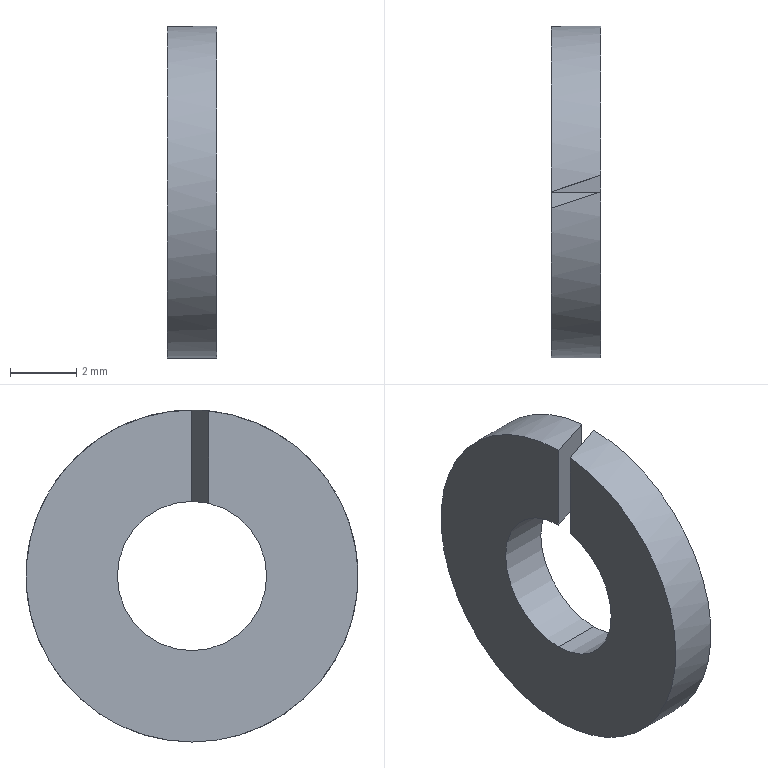Part | STEP file | 0244_Z_019_SCBZ6-25_2 | 1 solid | 8 faces | box 1.5 x 10 x 10 mm | volume 91.887 mm3 | cylinder 4 | plane 4 | commonest cylinder face diameters 4.5 x2 10 x2
STEP:
#1=CARTESIAN_POINT('',(0.,0.,0.));
#2=DIRECTION('',(0.,0.,1.));
#3=DIRECTION('',(1.,0.,0.));
#4=AXIS2_PLACEMENT_3D('',#1,#2,#3);
#5=CARTESIAN_POINT('',(0.,0.,-5.));
#6=VERTEX_POINT('',#5);
#7=CARTESIAN_POINT('',(0.,-0.5,4.975));
#8=VERTEX_POINT('',#7);
#9=CARTESIAN_POINT('',(0.,0.,0.));
#10=DIRECTION('',(-1.,0.,0.));
#11=DIRECTION('',(0.,0.,1.));
#12=AXIS2_PLACEMENT_3D('',#9,#10,#11);
#13=CIRCLE('',#12,5.);
#14=CARTESIAN_POINT('',(0.,0.,0.));
#15=DIRECTION('',(1.,0.,0.));
#16=DIRECTION('',(0.,0.,-1.));
#17=AXIS2_PLACEMENT_3D('',#14,#15,#16);
#18=CYLINDRICAL_SURFACE('',#17,5.);
#19=CARTESIAN_POINT('',(9.425,0.));
#20=DIRECTION('',(-1.,0.));
#21=VECTOR('',#20,1.);
#22=LINE('',#19,#21);
#23=(GEOMETRIC_REPRESENTATION_CONTEXT(2)PARAMETRIC_REPRESENTATION_CONTEXT()REPRESENTATION_CONTEXT('',''));
#24=DEFINITIONAL_REPRESENTATION('',(#22),#23);
#25=PCURVE('',#18,#24);
#26=CARTESIAN_POINT('',(0.,4.,0.));
#27=DIRECTION('',(-1.,0.,0.));
#28=DIRECTION('',(0.,0.,1.));
#29=AXIS2_PLACEMENT_3D('',#26,#27,#28);
#30=PLANE('',#29);
#31=CARTESIAN_POINT('',(0.,-4.));
#32=DIRECTION('',(1.,0.));
#33=AXIS2_PLACEMENT_2D('',#31,#32);
#34=CIRCLE('',#33,5.);
#35=(GEOMETRIC_REPRESENTATION_CONTEXT(2)PARAMETRIC_REPRESENTATION_CONTEXT()REPRESENTATION_CONTEXT('',''));
#36=DEFINITIONAL_REPRESENTATION('',(#34),#35);
#37=PCURVE('',#30,#36);
#38=SURFACE_CURVE('',#13,(#25,#37),.PCURVE_S1.);
#39=EDGE_CURVE('',#6,#8,#38,.T.);
#40=ORIENTED_EDGE('',*,*,#39,.F.);
#41=CARTESIAN_POINT('',(1.5,0.,-5.));
#42=VERTEX_POINT('',#41);
#43=CARTESIAN_POINT('',(0.,0.,-5.));
#44=DIRECTION('',(1.,0.,0.));
#45=VECTOR('',#44,1.);
#46=LINE('',#43,#45);
#47=CARTESIAN_POINT('',(6.283,0.));
#48=DIRECTION('',(0.,1.));
#49=VECTOR('',#48,1.);
#50=LINE('',#47,#49);
#51=(GEOMETRIC_REPRESENTATION_CONTEXT(2)PARAMETRIC_REPRESENTATION_CONTEXT()REPRESENTATION_CONTEXT('',''));
#52=DEFINITIONAL_REPRESENTATION('',(#50),#51);
#53=PCURVE('',#18,#52);
#54=CARTESIAN_POINT('',(0.,0.,0.));
#55=DIRECTION('',(1.,0.,0.));
#56=DIRECTION('',(0.,0.,-1.));
#57=AXIS2_PLACEMENT_3D('',#54,#55,#56);
#58=CYLINDRICAL_SURFACE('',#57,5.);
#59=CARTESIAN_POINT('',(0.,0.));
#60=DIRECTION('',(0.,1.));
#61=VECTOR('',#60,1.);
#62=LINE('',#59,#61);
#63=(GEOMETRIC_REPRESENTATION_CONTEXT(2)PARAMETRIC_REPRESENTATION_CONTEXT()REPRESENTATION_CONTEXT('',''));
#64=DEFINITIONAL_REPRESENTATION('',(#62),#63);
#65=PCURVE('',#58,#64);
#66=SURFACE_CURVE('',#46,(#53,#65),.PCURVE_S1.);
#67=EDGE_CURVE('',#6,#42,#66,.T.);
#68=ORIENTED_EDGE('',*,*,#67,.T.);
#69=CARTESIAN_POINT('',(1.5,0.,5.));
#70=VERTEX_POINT('',#69);
#71=CARTESIAN_POINT('',(1.5,0.,0.));
#72=DIRECTION('',(1.,0.,0.));
#73=DIRECTION('',(0.,0.,-1.));
#74=AXIS2_PLACEMENT_3D('',#71,#72,#73);
#75=CIRCLE('',#74,5.);
#76=CARTESIAN_POINT('',(0.,1.5));
#77=DIRECTION('',(1.,0.));
#78=VECTOR('',#77,1.);
#79=LINE('',#76,#78);
#80=(GEOMETRIC_REPRESENTATION_CONTEXT(2)PARAMETRIC_REPRESENTATION_CONTEXT()REPRESENTATION_CONTEXT('',''));
#81=DEFINITIONAL_REPRESENTATION('',(#79),#80);
#82=PCURVE('',#18,#81);
#83=CARTESIAN_POINT('',(1.5,4.,0.));
#84=DIRECTION('',(1.,0.,0.));
#85=DIRECTION('',(0.,0.,-1.));
#86=AXIS2_PLACEMENT_3D('',#83,#84,#85);
#87=PLANE('',#86);
#88=CARTESIAN_POINT('',(0.,-4.));
#89=DIRECTION('',(1.,0.));
#90=AXIS2_PLACEMENT_2D('',#88,#89);
#91=CIRCLE('',#90,5.);
#92=(GEOMETRIC_REPRESENTATION_CONTEXT(2)PARAMETRIC_REPRESENTATION_CONTEXT()REPRESENTATION_CONTEXT('',''));
#93=DEFINITIONAL_REPRESENTATION('',(#91),#92);
#94=PCURVE('',#87,#93);
#95=SURFACE_CURVE('',#75,(#82,#94),.PCURVE_S1.);
#96=EDGE_CURVE('',#70,#42,#95,.T.);
#97=ORIENTED_EDGE('',*,*,#96,.F.);
#98=CARTESIAN_POINT('',(1.5,0.,5.));
#99=CARTESIAN_POINT('',(0.999,-0.167,5.));
#100=CARTESIAN_POINT('',(0.4985,-0.3338,4.992));
#101=CARTESIAN_POINT('',(0.,-0.5,4.975));
#102=(BOUNDED_CURVE()B_SPLINE_CURVE(3,(#98,#99,#100,#101),.UNSPECIFIED.,.F.,.F.)B_SPLINE_CURVE_WITH_KNOTS((4,4),(1.571,1.671),.PIECEWISE_BEZIER_KNOTS.)CURVE()GEOMETRIC_REPRESENTATION_ITEM()RATIONAL_B_SPLINE_CURVE((1.,0.9992,0.9992,1.))REPRESENTATION_ITEM(''));
#103=CARTESIAN_POINT('',(3.142,1.5));
#104=CARTESIAN_POINT('',(3.143,1.477));
#105=CARTESIAN_POINT('',(3.146,1.432));
#106=CARTESIAN_POINT('',(3.151,1.363));
#107=CARTESIAN_POINT('',(3.155,1.295));
#108=CARTESIAN_POINT('',(3.16,1.227));
#109=CARTESIAN_POINT('',(3.164,1.159));
#110=CARTESIAN_POINT('',(3.169,1.09));
#111=CARTESIAN_POINT('',(3.173,1.022));
#112=CARTESIAN_POINT('',(3.178,0.9538));
#113=CARTESIAN_POINT('',(3.183,0.8855));
#114=CARTESIAN_POINT('',(3.187,0.8173));
#115=CARTESIAN_POINT('',(3.192,0.7491));
#116=CARTESIAN_POINT('',(3.196,0.6808));
#117=CARTESIAN_POINT('',(3.201,0.6126));
#118=CARTESIAN_POINT('',(3.205,0.5445));
#119=CARTESIAN_POINT('',(3.21,0.4763));
#120=CARTESIAN_POINT('',(3.214,0.4082));
#121=CARTESIAN_POINT('',(3.219,0.3401));
#122=CARTESIAN_POINT('',(3.224,0.272));
#123=CARTESIAN_POINT('',(3.228,0.2039));
#124=CARTESIAN_POINT('',(3.233,0.1359));
#125=CARTESIAN_POINT('',(3.237,0.06794));
#126=CARTESIAN_POINT('',(3.24,0.02264));
#127=CARTESIAN_POINT('',(3.242,0.));
#128=B_SPLINE_CURVE_WITH_KNOTS('',3,(#103,#104,#105,#106,#107,#108,#109,#110,#111,#112,#113,#114,#115,#116,#117,#118,#119,#120,#121,#122,#123,#124,#125,#126,#127),.UNSPECIFIED.,.F.,.F.,(4,1,1,1,1,1,1,1,1,1,1,1,1,1,1,1,1,1,1,1,1,1,4),(1.571,1.575,1.58,1.584,1.589,1.594,1.598,1.603,1.607,1.612,1.616,1.621,1.625,1.63,1.635,1.639,1.644,1.648,1.653,1.657,1.662,1.666,1.671),.QUASI_UNIFORM_KNOTS.);
#129=(GEOMETRIC_REPRESENTATION_CONTEXT(2)PARAMETRIC_REPRESENTATION_CONTEXT()REPRESENTATION_CONTEXT('',''));
#130=DEFINITIONAL_REPRESENTATION('',(#128),#129);
#131=PCURVE('',#18,#130);
#132=CARTESIAN_POINT('',(1.5,0.,0.));
#133=DIRECTION('',(0.3162,-0.9487,0.));
#134=DIRECTION('',(0.9487,0.3162,0.));
#135=AXIS2_PLACEMENT_3D('',#132,#133,#134);
#136=PLANE('',#135);
#137=CARTESIAN_POINT('',(0.,5.));
#138=CARTESIAN_POINT('',(-0.5281,5.));
#139=CARTESIAN_POINT('',(-1.056,4.992));
#140=CARTESIAN_POINT('',(-1.581,4.975));
#141=(BOUNDED_CURVE()B_SPLINE_CURVE(3,(#137,#138,#139,#140),.UNSPECIFIED.,.F.,.F.)B_SPLINE_CURVE_WITH_KNOTS((4,4),(1.571,1.671),.PIECEWISE_BEZIER_KNOTS.)CURVE()GEOMETRIC_REPRESENTATION_ITEM()RATIONAL_B_SPLINE_CURVE((1.,0.9992,0.9992,1.))REPRESENTATION_ITEM(''));
#142=(GEOMETRIC_REPRESENTATION_CONTEXT(2)PARAMETRIC_REPRESENTATION_CONTEXT()REPRESENTATION_CONTEXT('',''));
#143=DEFINITIONAL_REPRESENTATION('',(#141),#142);
#144=PCURVE('',#136,#143);
#145=SURFACE_CURVE('',#102,(#131,#144),.PCURVE_S1.);
#146=EDGE_CURVE('',#70,#8,#145,.T.);
#147=ORIENTED_EDGE('',*,*,#146,.T.);
#148=EDGE_LOOP('',(#40,#68,#97,#147));
#149=FACE_BOUND('',#148,.T.);
#150=ADVANCED_FACE('',(#149),#18,.T.);
#151=CARTESIAN_POINT('',(1.5,0.5,2.194));
#152=VERTEX_POINT('',#151);
#153=CARTESIAN_POINT('',(0.,0.,2.25));
#154=VERTEX_POINT('',#153);
#155=CARTESIAN_POINT('',(1.5,0.5,2.194));
#156=CARTESIAN_POINT('',(1.007,0.3358,2.231));
#157=CARTESIAN_POINT('',(0.5053,0.1684,2.25));
#158=CARTESIAN_POINT('',(0.,0.,2.25));
#159=(BOUNDED_CURVE()B_SPLINE_CURVE(3,(#155,#156,#157,#158),.UNSPECIFIED.,.F.,.F.)B_SPLINE_CURVE_WITH_KNOTS((4,4),(1.347,1.571),.PIECEWISE_BEZIER_KNOTS.)CURVE()GEOMETRIC_REPRESENTATION_ITEM()RATIONAL_B_SPLINE_CURVE((1.,0.9958,0.9958,1.))REPRESENTATION_ITEM(''));
#160=CARTESIAN_POINT('',(0.75,0.,0.));
#161=DIRECTION('',(1.,0.,0.));
#162=DIRECTION('',(0.,0.,-1.));
#163=AXIS2_PLACEMENT_3D('',#160,#161,#162);
#164=CYLINDRICAL_SURFACE('',#163,2.25);
#165=CARTESIAN_POINT('',(2.917,0.75));
#166=CARTESIAN_POINT('',(2.921,0.7277));
#167=CARTESIAN_POINT('',(2.928,0.683));
#168=CARTESIAN_POINT('',(2.938,0.6159));
#169=CARTESIAN_POINT('',(2.948,0.5485));
#170=CARTESIAN_POINT('',(2.958,0.481));
#171=CARTESIAN_POINT('',(2.968,0.4133));
#172=CARTESIAN_POINT('',(2.979,0.3455));
#173=CARTESIAN_POINT('',(2.989,0.2776));
#174=CARTESIAN_POINT('',(2.999,0.2095));
#175=CARTESIAN_POINT('',(3.009,0.1414));
#176=CARTESIAN_POINT('',(3.019,0.0731));
#177=CARTESIAN_POINT('',(3.03,0.004746));
#178=CARTESIAN_POINT('',(3.04,-0.06369));
#179=CARTESIAN_POINT('',(3.05,-0.1322));
#180=CARTESIAN_POINT('',(3.06,-0.2008));
#181=CARTESIAN_POINT('',(3.07,-0.2694));
#182=CARTESIAN_POINT('',(3.081,-0.338));
#183=CARTESIAN_POINT('',(3.091,-0.4067));
#184=CARTESIAN_POINT('',(3.101,-0.4754));
#185=CARTESIAN_POINT('',(3.111,-0.544));
#186=CARTESIAN_POINT('',(3.121,-0.6127));
#187=CARTESIAN_POINT('',(3.131,-0.6814));
#188=CARTESIAN_POINT('',(3.138,-0.7271));
#189=CARTESIAN_POINT('',(3.142,-0.75));
#190=B_SPLINE_CURVE_WITH_KNOTS('',3,(#165,#166,#167,#168,#169,#170,#171,#172,#173,#174,#175,#176,#177,#178,#179,#180,#181,#182,#183,#184,#185,#186,#187,#188,#189),.UNSPECIFIED.,.F.,.F.,(4,1,1,1,1,1,1,1,1,1,1,1,1,1,1,1,1,1,1,1,1,1,4),(1.347,1.357,1.367,1.377,1.387,1.398,1.408,1.418,1.428,1.438,1.449,1.459,1.469,1.479,1.489,1.499,1.51,1.52,1.53,1.54,1.55,1.561,1.571),.QUASI_UNIFORM_KNOTS.);
#191=(GEOMETRIC_REPRESENTATION_CONTEXT(2)PARAMETRIC_REPRESENTATION_CONTEXT()REPRESENTATION_CONTEXT('',''));
#192=DEFINITIONAL_REPRESENTATION('',(#190),#191);
#193=PCURVE('',#164,#192);
#194=CARTESIAN_POINT('',(0.,0.,0.));
#195=DIRECTION('',(-0.3162,0.9487,0.));
#196=DIRECTION('',(-0.9487,-0.3162,0.));
#197=AXIS2_PLACEMENT_3D('',#194,#195,#196);
#198=PLANE('',#197);
#199=CARTESIAN_POINT('',(-1.581,2.194));
#200=CARTESIAN_POINT('',(-1.062,2.231));
#201=CARTESIAN_POINT('',(-0.5326,2.25));
#202=CARTESIAN_POINT('',(0.,2.25));
#203=(BOUNDED_CURVE()B_SPLINE_CURVE(3,(#199,#200,#201,#202),.UNSPECIFIED.,.F.,.F.)B_SPLINE_CURVE_WITH_KNOTS((4,4),(1.347,1.571),.PIECEWISE_BEZIER_KNOTS.)CURVE()GEOMETRIC_REPRESENTATION_ITEM()RATIONAL_B_SPLINE_CURVE((1.,0.9958,0.9958,1.))REPRESENTATION_ITEM(''));
#204=(GEOMETRIC_REPRESENTATION_CONTEXT(2)PARAMETRIC_REPRESENTATION_CONTEXT()REPRESENTATION_CONTEXT('',''));
#205=DEFINITIONAL_REPRESENTATION('',(#203),#204);
#206=PCURVE('',#198,#205);
#207=SURFACE_CURVE('',#159,(#193,#206),.PCURVE_S1.);
#208=EDGE_CURVE('',#152,#154,#207,.T.);
#209=ORIENTED_EDGE('',*,*,#208,.F.);
#210=CARTESIAN_POINT('',(1.5,0.,-2.25));
#211=VERTEX_POINT('',#210);
#212=CARTESIAN_POINT('',(1.5,0.,0.));
#213=DIRECTION('',(-1.,0.,0.));
#214=DIRECTION('',(0.,0.,-1.));
#215=AXIS2_PLACEMENT_3D('',#212,#213,#214);
#216=CIRCLE('',#215,2.25);
#217=CARTESIAN_POINT('',(6.283,0.75));
#218=DIRECTION('',(-1.,0.));
#219=VECTOR('',#218,1.);
#220=LINE('',#217,#219);
#221=(GEOMETRIC_REPRESENTATION_CONTEXT(2)PARAMETRIC_REPRESENTATION_CONTEXT()REPRESENTATION_CONTEXT('',''));
#222=DEFINITIONAL_REPRESENTATION('',(#220),#221);
#223=PCURVE('',#164,#222);
#224=CARTESIAN_POINT('',(2.25,-4.));
#225=CARTESIAN_POINT('',(2.25,-7.897));
#226=CARTESIAN_POINT('',(-1.125,-5.949));
#227=CARTESIAN_POINT('',(-4.5,-4.));
#228=CARTESIAN_POINT('',(-1.125,-2.051));
#229=CARTESIAN_POINT('',(2.25,-0.1029));
#230=CARTESIAN_POINT('',(2.25,-4.));
#231=(BOUNDED_CURVE()B_SPLINE_CURVE(2,(#224,#225,#226,#227,#228,#229,#230),.UNSPECIFIED.,.T.,.F.)B_SPLINE_CURVE_WITH_KNOTS((1,2,2,2,2,1),(-2.094,0.,2.094,4.189,6.283,8.378),.UNSPECIFIED.)CURVE()GEOMETRIC_REPRESENTATION_ITEM()RATIONAL_B_SPLINE_CURVE((1.,0.5,1.,0.5,1.,0.5,1.))REPRESENTATION_ITEM(''));
#232=(GEOMETRIC_REPRESENTATION_CONTEXT(2)PARAMETRIC_REPRESENTATION_CONTEXT()REPRESENTATION_CONTEXT('',''));
#233=DEFINITIONAL_REPRESENTATION('',(#231),#232);
#234=PCURVE('',#87,#233);
#235=SURFACE_CURVE('',#216,(#223,#234),.PCURVE_S1.);
#236=EDGE_CURVE('',#152,#211,#235,.T.);
#237=ORIENTED_EDGE('',*,*,#236,.T.);
#238=CARTESIAN_POINT('',(0.,0.,-2.25));
#239=VERTEX_POINT('',#238);
#240=CARTESIAN_POINT('',(0.75,0.,-2.25));
#241=DIRECTION('',(1.,0.,0.));
#242=VECTOR('',#241,1.);
#243=LINE('',#240,#242);
#244=CARTESIAN_POINT('',(0.,0.));
#245=DIRECTION('',(0.,1.));
#246=VECTOR('',#245,1.);
#247=LINE('',#244,#246);
#248=(GEOMETRIC_REPRESENTATION_CONTEXT(2)PARAMETRIC_REPRESENTATION_CONTEXT()REPRESENTATION_CONTEXT('',''));
#249=DEFINITIONAL_REPRESENTATION('',(#247),#248);
#250=PCURVE('',#164,#249);
#251=CARTESIAN_POINT('',(0.75,0.,0.));
#252=DIRECTION('',(1.,0.,0.));
#253=DIRECTION('',(0.,0.,-1.));
#254=AXIS2_PLACEMENT_3D('',#251,#252,#253);
#255=CYLINDRICAL_SURFACE('',#254,2.25);
#256=CARTESIAN_POINT('',(6.283,0.));
#257=DIRECTION('',(0.,1.));
#258=VECTOR('',#257,1.);
#259=LINE('',#256,#258);
#260=(GEOMETRIC_REPRESENTATION_CONTEXT(2)PARAMETRIC_REPRESENTATION_CONTEXT()REPRESENTATION_CONTEXT('',''));
#261=DEFINITIONAL_REPRESENTATION('',(#259),#260);
#262=PCURVE('',#255,#261);
#263=SURFACE_CURVE('',#243,(#250,#262),.PCURVE_S1.);
#264=EDGE_CURVE('',#239,#211,#263,.T.);
#265=ORIENTED_EDGE('',*,*,#264,.F.);
#266=CARTESIAN_POINT('',(0.,0.,0.));
#267=DIRECTION('',(1.,0.,0.));
#268=DIRECTION('',(0.,0.,-1.));
#269=AXIS2_PLACEMENT_3D('',#266,#267,#268);
#270=CIRCLE('',#269,2.25);
#271=CARTESIAN_POINT('',(0.,-0.75));
#272=DIRECTION('',(1.,0.));
#273=VECTOR('',#272,1.);
#274=LINE('',#271,#273);
#275=(GEOMETRIC_REPRESENTATION_CONTEXT(2)PARAMETRIC_REPRESENTATION_CONTEXT()REPRESENTATION_CONTEXT('',''));
#276=DEFINITIONAL_REPRESENTATION('',(#274),#275);
#277=PCURVE('',#164,#276);
#278=CARTESIAN_POINT('',(-2.25,-4.));
#279=CARTESIAN_POINT('',(-2.25,-0.1029));
#280=CARTESIAN_POINT('',(1.125,-2.051));
#281=CARTESIAN_POINT('',(4.5,-4.));
#282=CARTESIAN_POINT('',(1.125,-5.949));
#283=CARTESIAN_POINT('',(-2.25,-7.897));
#284=CARTESIAN_POINT('',(-2.25,-4.));
#285=(BOUNDED_CURVE()B_SPLINE_CURVE(2,(#278,#279,#280,#281,#282,#283,#284),.UNSPECIFIED.,.T.,.F.)B_SPLINE_CURVE_WITH_KNOTS((1,2,2,2,2,1),(-2.094,0.,2.094,4.189,6.283,8.378),.UNSPECIFIED.)CURVE()GEOMETRIC_REPRESENTATION_ITEM()RATIONAL_B_SPLINE_CURVE((1.,0.5,1.,0.5,1.,0.5,1.))REPRESENTATION_ITEM(''));
#286=(GEOMETRIC_REPRESENTATION_CONTEXT(2)PARAMETRIC_REPRESENTATION_CONTEXT()REPRESENTATION_CONTEXT('',''));
#287=DEFINITIONAL_REPRESENTATION('',(#285),#286);
#288=PCURVE('',#30,#287);
#289=SURFACE_CURVE('',#270,(#277,#288),.PCURVE_S1.);
#290=EDGE_CURVE('',#239,#154,#289,.T.);
#291=ORIENTED_EDGE('',*,*,#290,.T.);
#292=EDGE_LOOP('',(#209,#237,#265,#291));
#293=FACE_BOUND('',#292,.F.);
#294=ADVANCED_FACE('',(#293),#164,.F.);
#295=CARTESIAN_POINT('',(1.5,0.,2.25));
#296=VERTEX_POINT('',#295);
#297=CARTESIAN_POINT('',(1.5,0.,0.));
#298=DIRECTION('',(0.,0.,1.));
#299=VECTOR('',#298,1.);
#300=LINE('',#297,#299);
#301=CARTESIAN_POINT('',(0.,-4.));
#302=DIRECTION('',(-1.,0.));
#303=VECTOR('',#302,1.);
#304=LINE('',#301,#303);
#305=(GEOMETRIC_REPRESENTATION_CONTEXT(2)PARAMETRIC_REPRESENTATION_CONTEXT()REPRESENTATION_CONTEXT('',''));
#306=DEFINITIONAL_REPRESENTATION('',(#304),#305);
#307=PCURVE('',#87,#306);
#308=CARTESIAN_POINT('',(0.,0.));
#309=DIRECTION('',(0.,1.));
#310=VECTOR('',#309,1.);
#311=LINE('',#308,#310);
#312=(GEOMETRIC_REPRESENTATION_CONTEXT(2)PARAMETRIC_REPRESENTATION_CONTEXT()REPRESENTATION_CONTEXT('',''));
#313=DEFINITIONAL_REPRESENTATION('',(#311),#312);
#314=PCURVE('',#136,#313);
#315=SURFACE_CURVE('',#300,(#307,#314),.PCURVE_S1.);
#316=EDGE_CURVE('',#296,#70,#315,.T.);
#317=ORIENTED_EDGE('',*,*,#316,.T.);
#318=ORIENTED_EDGE('',*,*,#96,.T.);
#319=CARTESIAN_POINT('',(1.5,0.5,4.975));
#320=VERTEX_POINT('',#319);
#321=CARTESIAN_POINT('',(1.5,0.,0.));
#322=DIRECTION('',(1.,0.,0.));
#323=DIRECTION('',(0.,0.,-1.));
#324=AXIS2_PLACEMENT_3D('',#321,#322,#323);
#325=CIRCLE('',#324,5.);
#326=CARTESIAN_POINT('',(0.,-4.));
#327=DIRECTION('',(1.,0.));
#328=AXIS2_PLACEMENT_2D('',#326,#327);
#329=CIRCLE('',#328,5.);
#330=(GEOMETRIC_REPRESENTATION_CONTEXT(2)PARAMETRIC_REPRESENTATION_CONTEXT()REPRESENTATION_CONTEXT('',''));
#331=DEFINITIONAL_REPRESENTATION('',(#329),#330);
#332=PCURVE('',#87,#331);
#333=CARTESIAN_POINT('',(0.,1.5));
#334=DIRECTION('',(1.,0.));
#335=VECTOR('',#334,1.);
#336=LINE('',#333,#335);
#337=(GEOMETRIC_REPRESENTATION_CONTEXT(2)PARAMETRIC_REPRESENTATION_CONTEXT()REPRESENTATION_CONTEXT('',''));
#338=DEFINITIONAL_REPRESENTATION('',(#336),#337);
#339=PCURVE('',#58,#338);
#340=SURFACE_CURVE('',#325,(#332,#339),.PCURVE_S1.);
#341=EDGE_CURVE('',#42,#320,#340,.T.);
#342=ORIENTED_EDGE('',*,*,#341,.T.);
#343=CARTESIAN_POINT('',(1.5,0.5,0.));
#344=DIRECTION('',(0.,0.,-1.));
#345=VECTOR('',#344,1.);
#346=LINE('',#343,#345);
#347=CARTESIAN_POINT('',(0.,-3.5));
#348=DIRECTION('',(1.,0.));
#349=VECTOR('',#348,1.);
#350=LINE('',#347,#349);
#351=(GEOMETRIC_REPRESENTATION_CONTEXT(2)PARAMETRIC_REPRESENTATION_CONTEXT()REPRESENTATION_CONTEXT('',''));
#352=DEFINITIONAL_REPRESENTATION('',(#350),#351);
#353=PCURVE('',#87,#352);
#354=CARTESIAN_POINT('',(-1.581,0.));
#355=DIRECTION('',(0.,-1.));
#356=VECTOR('',#355,1.);
#357=LINE('',#354,#356);
#358=(GEOMETRIC_REPRESENTATION_CONTEXT(2)PARAMETRIC_REPRESENTATION_CONTEXT()REPRESENTATION_CONTEXT('',''));
#359=DEFINITIONAL_REPRESENTATION('',(#357),#358);
#360=PCURVE('',#198,#359);
#361=SURFACE_CURVE('',#346,(#353,#360),.PCURVE_S1.);
#362=EDGE_CURVE('',#320,#152,#361,.T.);
#363=ORIENTED_EDGE('',*,*,#362,.T.);
#364=ORIENTED_EDGE('',*,*,#236,.T.);
#365=CARTESIAN_POINT('',(1.5,0.,0.));
#366=DIRECTION('',(-1.,0.,0.));
#367=DIRECTION('',(0.,0.,-1.));
#368=AXIS2_PLACEMENT_3D('',#365,#366,#367);
#369=CIRCLE('',#368,2.25);
#370=CARTESIAN_POINT('',(2.25,-4.));
#371=CARTESIAN_POINT('',(2.25,-7.897));
#372=CARTESIAN_POINT('',(-1.125,-5.949));
#373=CARTESIAN_POINT('',(-4.5,-4.));
#374=CARTESIAN_POINT('',(-1.125,-2.051));
#375=CARTESIAN_POINT('',(2.25,-0.1029));
#376=CARTESIAN_POINT('',(2.25,-4.));
#377=(BOUNDED_CURVE()B_SPLINE_CURVE(2,(#370,#371,#372,#373,#374,#375,#376),.UNSPECIFIED.,.T.,.F.)B_SPLINE_CURVE_WITH_KNOTS((1,2,2,2,2,1),(-2.094,0.,2.094,4.189,6.283,8.378),.UNSPECIFIED.)CURVE()GEOMETRIC_REPRESENTATION_ITEM()RATIONAL_B_SPLINE_CURVE((1.,0.5,1.,0.5,1.,0.5,1.))REPRESENTATION_ITEM(''));
#378=(GEOMETRIC_REPRESENTATION_CONTEXT(2)PARAMETRIC_REPRESENTATION_CONTEXT()REPRESENTATION_CONTEXT('',''));
#379=DEFINITIONAL_REPRESENTATION('',(#377),#378);
#380=PCURVE('',#87,#379);
#381=CARTESIAN_POINT('',(6.283,0.75));
#382=DIRECTION('',(-1.,0.));
#383=VECTOR('',#382,1.);
#384=LINE('',#381,#383);
#385=(GEOMETRIC_REPRESENTATION_CONTEXT(2)PARAMETRIC_REPRESENTATION_CONTEXT()REPRESENTATION_CONTEXT('',''));
#386=DEFINITIONAL_REPRESENTATION('',(#384),#385);
#387=PCURVE('',#255,#386);
#388=SURFACE_CURVE('',#369,(#380,#387),.PCURVE_S1.);
#389=EDGE_CURVE('',#211,#296,#388,.T.);
#390=ORIENTED_EDGE('',*,*,#389,.T.);
#391=EDGE_LOOP('',(#317,#318,#342,#363,#364,#390));
#392=FACE_BOUND('',#391,.T.);
#393=ADVANCED_FACE('',(#392),#87,.T.);
#394=ORIENTED_EDGE('',*,*,#146,.F.);
#395=ORIENTED_EDGE('',*,*,#316,.F.);
#396=CARTESIAN_POINT('',(0.,-0.5,2.194));
#397=VERTEX_POINT('',#396);
#398=CARTESIAN_POINT('',(1.5,0.,2.25));
#399=CARTESIAN_POINT('',(0.9947,-0.1684,2.25));
#400=CARTESIAN_POINT('',(0.4926,-0.3358,2.231));
#401=CARTESIAN_POINT('',(0.,-0.5,2.194));
#402=(BOUNDED_CURVE()B_SPLINE_CURVE(3,(#398,#399,#400,#401),.UNSPECIFIED.,.F.,.F.)B_SPLINE_CURVE_WITH_KNOTS((4,4),(1.571,1.795),.PIECEWISE_BEZIER_KNOTS.)CURVE()GEOMETRIC_REPRESENTATION_ITEM()RATIONAL_B_SPLINE_CURVE((1.,0.9958,0.9958,1.))REPRESENTATION_ITEM(''));
#403=CARTESIAN_POINT('',(0.,2.25));
#404=CARTESIAN_POINT('',(-0.5326,2.25));
#405=CARTESIAN_POINT('',(-1.062,2.231));
#406=CARTESIAN_POINT('',(-1.581,2.194));
#407=(BOUNDED_CURVE()B_SPLINE_CURVE(3,(#403,#404,#405,#406),.UNSPECIFIED.,.F.,.F.)B_SPLINE_CURVE_WITH_KNOTS((4,4),(1.571,1.795),.PIECEWISE_BEZIER_KNOTS.)CURVE()GEOMETRIC_REPRESENTATION_ITEM()RATIONAL_B_SPLINE_CURVE((1.,0.9958,0.9958,1.))REPRESENTATION_ITEM(''));
#408=(GEOMETRIC_REPRESENTATION_CONTEXT(2)PARAMETRIC_REPRESENTATION_CONTEXT()REPRESENTATION_CONTEXT('',''));
#409=DEFINITIONAL_REPRESENTATION('',(#407),#408);
#410=PCURVE('',#136,#409);
#411=CARTESIAN_POINT('',(3.142,0.75));
#412=CARTESIAN_POINT('',(3.145,0.7271));
#413=CARTESIAN_POINT('',(3.152,0.6814));
#414=CARTESIAN_POINT('',(3.162,0.6127));
#415=CARTESIAN_POINT('',(3.172,0.544));
#416=CARTESIAN_POINT('',(3.182,0.4754));
#417=CARTESIAN_POINT('',(3.192,0.4067));
#418=CARTESIAN_POINT('',(3.203,0.338));
#419=CARTESIAN_POINT('',(3.213,0.2694));
#420=CARTESIAN_POINT('',(3.223,0.2008));
#421=CARTESIAN_POINT('',(3.233,0.1322));
#422=CARTESIAN_POINT('',(3.243,0.06369));
#423=CARTESIAN_POINT('',(3.254,-0.004746));
#424=CARTESIAN_POINT('',(3.264,-0.0731));
#425=CARTESIAN_POINT('',(3.274,-0.1414));
#426=CARTESIAN_POINT('',(3.284,-0.2095));
#427=CARTESIAN_POINT('',(3.294,-0.2776));
#428=CARTESIAN_POINT('',(3.305,-0.3455));
#429=CARTESIAN_POINT('',(3.315,-0.4133));
#430=CARTESIAN_POINT('',(3.325,-0.481));
#431=CARTESIAN_POINT('',(3.335,-0.5485));
#432=CARTESIAN_POINT('',(3.345,-0.6159));
#433=CARTESIAN_POINT('',(3.356,-0.683));
#434=CARTESIAN_POINT('',(3.362,-0.7277));
#435=CARTESIAN_POINT('',(3.366,-0.75));
#436=B_SPLINE_CURVE_WITH_KNOTS('',3,(#411,#412,#413,#414,#415,#416,#417,#418,#419,#420,#421,#422,#423,#424,#425,#426,#427,#428,#429,#430,#431,#432,#433,#434,#435),.UNSPECIFIED.,.F.,.F.,(4,1,1,1,1,1,1,1,1,1,1,1,1,1,1,1,1,1,1,1,1,1,4),(1.571,1.581,1.591,1.601,1.612,1.622,1.632,1.642,1.652,1.662,1.673,1.683,1.693,1.703,1.713,1.724,1.734,1.744,1.754,1.764,1.775,1.785,1.795),.QUASI_UNIFORM_KNOTS.);
#437=(GEOMETRIC_REPRESENTATION_CONTEXT(2)PARAMETRIC_REPRESENTATION_CONTEXT()REPRESENTATION_CONTEXT('',''));
#438=DEFINITIONAL_REPRESENTATION('',(#436),#437);
#439=PCURVE('',#255,#438);
#440=SURFACE_CURVE('',#402,(#410,#439),.PCURVE_S1.);
#441=EDGE_CURVE('',#296,#397,#440,.T.);
#442=ORIENTED_EDGE('',*,*,#441,.T.);
#443=CARTESIAN_POINT('',(0.,-0.5,0.));
#444=DIRECTION('',(0.,0.,-1.));
#445=VECTOR('',#444,1.);
#446=LINE('',#443,#445);
#447=CARTESIAN_POINT('',(-1.581,0.));
#448=DIRECTION('',(0.,-1.));
#449=VECTOR('',#448,1.);
#450=LINE('',#447,#449);
#451=(GEOMETRIC_REPRESENTATION_CONTEXT(2)PARAMETRIC_REPRESENTATION_CONTEXT()REPRESENTATION_CONTEXT('',''));
#452=DEFINITIONAL_REPRESENTATION('',(#450),#451);
#453=PCURVE('',#136,#452);
#454=CARTESIAN_POINT('',(0.,-4.5));
#455=DIRECTION('',(-1.,0.));
#456=VECTOR('',#455,1.);
#457=LINE('',#454,#456);
#458=(GEOMETRIC_REPRESENTATION_CONTEXT(2)PARAMETRIC_REPRESENTATION_CONTEXT()REPRESENTATION_CONTEXT('',''));
#459=DEFINITIONAL_REPRESENTATION('',(#457),#458);
#460=PCURVE('',#30,#459);
#461=SURFACE_CURVE('',#446,(#453,#460),.PCURVE_S1.);
#462=EDGE_CURVE('',#8,#397,#461,.T.);
#463=ORIENTED_EDGE('',*,*,#462,.F.);
#464=EDGE_LOOP('',(#394,#395,#442,#463));
#465=FACE_BOUND('',#464,.T.);
#466=ADVANCED_FACE('',(#465),#136,.F.);
#467=CARTESIAN_POINT('',(0.,0.,5.));
#468=VERTEX_POINT('',#467);
#469=CARTESIAN_POINT('',(0.,0.,5.));
#470=CARTESIAN_POINT('',(0.501,0.167,5.));
#471=CARTESIAN_POINT('',(1.001,0.3338,4.992));
#472=CARTESIAN_POINT('',(1.5,0.5,4.975));
#473=(BOUNDED_CURVE()B_SPLINE_CURVE(3,(#469,#470,#471,#472),.UNSPECIFIED.,.F.,.F.)B_SPLINE_CURVE_WITH_KNOTS((4,4),(4.712,4.813),.PIECEWISE_BEZIER_KNOTS.)CURVE()GEOMETRIC_REPRESENTATION_ITEM()RATIONAL_B_SPLINE_CURVE((1.,0.9992,0.9992,1.))REPRESENTATION_ITEM(''));
#474=CARTESIAN_POINT('',(0.,5.));
#475=CARTESIAN_POINT('',(-0.5281,5.));
#476=CARTESIAN_POINT('',(-1.056,4.992));
#477=CARTESIAN_POINT('',(-1.581,4.975));
#478=(BOUNDED_CURVE()B_SPLINE_CURVE(3,(#474,#475,#476,#477),.UNSPECIFIED.,.F.,.F.)B_SPLINE_CURVE_WITH_KNOTS((4,4),(4.712,4.813),.PIECEWISE_BEZIER_KNOTS.)CURVE()GEOMETRIC_REPRESENTATION_ITEM()RATIONAL_B_SPLINE_CURVE((1.,0.9992,0.9992,1.))REPRESENTATION_ITEM(''));
#479=(GEOMETRIC_REPRESENTATION_CONTEXT(2)PARAMETRIC_REPRESENTATION_CONTEXT()REPRESENTATION_CONTEXT('',''));
#480=DEFINITIONAL_REPRESENTATION('',(#478),#479);
#481=PCURVE('',#198,#480);
#482=CARTESIAN_POINT('',(3.142,0.));
#483=CARTESIAN_POINT('',(3.14,0.02276));
#484=CARTESIAN_POINT('',(3.137,0.06827));
#485=CARTESIAN_POINT('',(3.132,0.1365));
#486=CARTESIAN_POINT('',(3.128,0.2048));
#487=CARTESIAN_POINT('',(3.123,0.2731));
#488=CARTESIAN_POINT('',(3.119,0.3414));
#489=CARTESIAN_POINT('',(3.114,0.4097));
#490=CARTESIAN_POINT('',(3.11,0.4779));
#491=CARTESIAN_POINT('',(3.105,0.5462));
#492=CARTESIAN_POINT('',(3.101,0.6145));
#493=CARTESIAN_POINT('',(3.096,0.6827));
#494=CARTESIAN_POINT('',(3.092,0.7509));
#495=CARTESIAN_POINT('',(3.087,0.8192));
#496=CARTESIAN_POINT('',(3.082,0.8874));
#497=CARTESIAN_POINT('',(3.078,0.9555));
#498=CARTESIAN_POINT('',(3.073,1.024));
#499=CARTESIAN_POINT('',(3.069,1.092));
#500=CARTESIAN_POINT('',(3.064,1.16));
#501=CARTESIAN_POINT('',(3.06,1.228));
#502=CARTESIAN_POINT('',(3.055,1.296));
#503=CARTESIAN_POINT('',(3.051,1.364));
#504=CARTESIAN_POINT('',(3.046,1.432));
#505=CARTESIAN_POINT('',(3.043,1.477));
#506=CARTESIAN_POINT('',(3.041,1.5));
#507=B_SPLINE_CURVE_WITH_KNOTS('',3,(#482,#483,#484,#485,#486,#487,#488,#489,#490,#491,#492,#493,#494,#495,#496,#497,#498,#499,#500,#501,#502,#503,#504,#505,#506),.UNSPECIFIED.,.F.,.F.,(4,1,1,1,1,1,1,1,1,1,1,1,1,1,1,1,1,1,1,1,1,1,4),(4.712,4.717,4.721,4.726,4.731,4.735,4.74,4.744,4.749,4.753,4.758,4.762,4.767,4.772,4.776,4.781,4.785,4.79,4.794,4.799,4.803,4.808,4.813),.QUASI_UNIFORM_KNOTS.);
#508=(GEOMETRIC_REPRESENTATION_CONTEXT(2)PARAMETRIC_REPRESENTATION_CONTEXT()REPRESENTATION_CONTEXT('',''));
#509=DEFINITIONAL_REPRESENTATION('',(#507),#508);
#510=PCURVE('',#58,#509);
#511=SURFACE_CURVE('',#473,(#481,#510),.PCURVE_S1.);
#512=EDGE_CURVE('',#468,#320,#511,.T.);
#513=ORIENTED_EDGE('',*,*,#512,.F.);
#514=CARTESIAN_POINT('',(0.,0.,0.));
#515=DIRECTION('',(0.,0.,1.));
#516=VECTOR('',#515,1.);
#517=LINE('',#514,#516);
#518=CARTESIAN_POINT('',(0.,0.));
#519=DIRECTION('',(0.,1.));
#520=VECTOR('',#519,1.);
#521=LINE('',#518,#520);
#522=(GEOMETRIC_REPRESENTATION_CONTEXT(2)PARAMETRIC_REPRESENTATION_CONTEXT()REPRESENTATION_CONTEXT('',''));
#523=DEFINITIONAL_REPRESENTATION('',(#521),#522);
#524=PCURVE('',#198,#523);
#525=CARTESIAN_POINT('',(0.,-4.));
#526=DIRECTION('',(1.,0.));
#527=VECTOR('',#526,1.);
#528=LINE('',#525,#527);
#529=(GEOMETRIC_REPRESENTATION_CONTEXT(2)PARAMETRIC_REPRESENTATION_CONTEXT()REPRESENTATION_CONTEXT('',''));
#530=DEFINITIONAL_REPRESENTATION('',(#528),#529);
#531=PCURVE('',#30,#530);
#532=SURFACE_CURVE('',#517,(#524,#531),.PCURVE_S1.);
#533=EDGE_CURVE('',#154,#468,#532,.T.);
#534=ORIENTED_EDGE('',*,*,#533,.F.);
#535=ORIENTED_EDGE('',*,*,#208,.F.);
#536=ORIENTED_EDGE('',*,*,#362,.F.);
#537=EDGE_LOOP('',(#513,#534,#535,#536));
#538=FACE_BOUND('',#537,.T.);
#539=ADVANCED_FACE('',(#538),#198,.F.);
#540=ORIENTED_EDGE('',*,*,#533,.T.);
#541=CARTESIAN_POINT('',(0.,0.,0.));
#542=DIRECTION('',(-1.,0.,0.));
#543=DIRECTION('',(0.,0.,1.));
#544=AXIS2_PLACEMENT_3D('',#541,#542,#543);
#545=CIRCLE('',#544,5.);
#546=CARTESIAN_POINT('',(0.,-4.));
#547=DIRECTION('',(1.,0.));
#548=AXIS2_PLACEMENT_2D('',#546,#547);
#549=CIRCLE('',#548,5.);
#550=(GEOMETRIC_REPRESENTATION_CONTEXT(2)PARAMETRIC_REPRESENTATION_CONTEXT()REPRESENTATION_CONTEXT('',''));
#551=DEFINITIONAL_REPRESENTATION('',(#549),#550);
#552=PCURVE('',#30,#551);
#553=CARTESIAN_POINT('',(3.142,0.));
#554=DIRECTION('',(-1.,0.));
#555=VECTOR('',#554,1.);
#556=LINE('',#553,#555);
#557=(GEOMETRIC_REPRESENTATION_CONTEXT(2)PARAMETRIC_REPRESENTATION_CONTEXT()REPRESENTATION_CONTEXT('',''));
#558=DEFINITIONAL_REPRESENTATION('',(#556),#557);
#559=PCURVE('',#58,#558);
#560=SURFACE_CURVE('',#545,(#552,#559),.PCURVE_S1.);
#561=EDGE_CURVE('',#468,#6,#560,.T.);
#562=ORIENTED_EDGE('',*,*,#561,.T.);
#563=ORIENTED_EDGE('',*,*,#39,.T.);
#564=ORIENTED_EDGE('',*,*,#462,.T.);
#565=CARTESIAN_POINT('',(0.,0.,0.));
#566=DIRECTION('',(1.,0.,0.));
#567=DIRECTION('',(0.,0.,-1.));
#568=AXIS2_PLACEMENT_3D('',#565,#566,#567);
#569=CIRCLE('',#568,2.25);
#570=CARTESIAN_POINT('',(-2.25,-4.));
#571=CARTESIAN_POINT('',(-2.25,-0.1029));
#572=CARTESIAN_POINT('',(1.125,-2.051));
#573=CARTESIAN_POINT('',(4.5,-4.));
#574=CARTESIAN_POINT('',(1.125,-5.949));
#575=CARTESIAN_POINT('',(-2.25,-7.897));
#576=CARTESIAN_POINT('',(-2.25,-4.));
#577=(BOUNDED_CURVE()B_SPLINE_CURVE(2,(#570,#571,#572,#573,#574,#575,#576),.UNSPECIFIED.,.T.,.F.)B_SPLINE_CURVE_WITH_KNOTS((1,2,2,2,2,1),(-2.094,0.,2.094,4.189,6.283,8.378),.UNSPECIFIED.)CURVE()GEOMETRIC_REPRESENTATION_ITEM()RATIONAL_B_SPLINE_CURVE((1.,0.5,1.,0.5,1.,0.5,1.))REPRESENTATION_ITEM(''));
#578=(GEOMETRIC_REPRESENTATION_CONTEXT(2)PARAMETRIC_REPRESENTATION_CONTEXT()REPRESENTATION_CONTEXT('',''));
#579=DEFINITIONAL_REPRESENTATION('',(#577),#578);
#580=PCURVE('',#30,#579);
#581=CARTESIAN_POINT('',(0.,-0.75));
#582=DIRECTION('',(1.,0.));
#583=VECTOR('',#582,1.);
#584=LINE('',#581,#583);
#585=(GEOMETRIC_REPRESENTATION_CONTEXT(2)PARAMETRIC_REPRESENTATION_CONTEXT()REPRESENTATION_CONTEXT('',''));
#586=DEFINITIONAL_REPRESENTATION('',(#584),#585);
#587=PCURVE('',#255,#586);
#588=SURFACE_CURVE('',#569,(#580,#587),.PCURVE_S1.);
#589=EDGE_CURVE('',#397,#239,#588,.T.);
#590=ORIENTED_EDGE('',*,*,#589,.T.);
#591=ORIENTED_EDGE('',*,*,#290,.T.);
#592=EDGE_LOOP('',(#540,#562,#563,#564,#590,#591));
#593=FACE_BOUND('',#592,.T.);
#594=ADVANCED_FACE('',(#593),#30,.T.);
#595=ORIENTED_EDGE('',*,*,#389,.T.);
#596=ORIENTED_EDGE('',*,*,#441,.T.);
#597=ORIENTED_EDGE('',*,*,#589,.T.);
#598=ORIENTED_EDGE('',*,*,#264,.T.);
#599=EDGE_LOOP('',(#595,#596,#597,#598));
#600=FACE_BOUND('',#599,.F.);
#601=ADVANCED_FACE('',(#600),#255,.F.);
#602=ORIENTED_EDGE('',*,*,#67,.F.);
#603=ORIENTED_EDGE('',*,*,#561,.F.);
#604=ORIENTED_EDGE('',*,*,#512,.T.);
#605=ORIENTED_EDGE('',*,*,#341,.F.);
#606=EDGE_LOOP('',(#602,#603,#604,#605));
#607=FACE_BOUND('',#606,.T.);
#608=ADVANCED_FACE('',(#607),#58,.T.);
#609=CLOSED_SHELL('',(#150,#294,#393,#466,#539,#594,#601,#608));
#610=MANIFOLD_SOLID_BREP('',#609);
#611=(LENGTH_UNIT()NAMED_UNIT(*)SI_UNIT(.MILLI.,.METRE.));
#612=UNCERTAINTY_MEASURE_WITH_UNIT(LENGTH_MEASURE(0.0000001),#611,'','');
#613=(NAMED_UNIT(*)PLANE_ANGLE_UNIT()SI_UNIT($,.RADIAN.));
#614=(NAMED_UNIT(*)SI_UNIT($,.STERADIAN.)SOLID_ANGLE_UNIT());
#615=(GEOMETRIC_REPRESENTATION_CONTEXT(3)GLOBAL_UNCERTAINTY_ASSIGNED_CONTEXT((#612))GLOBAL_UNIT_ASSIGNED_CONTEXT((#611,#613,#614))REPRESENTATION_CONTEXT('',''));
#616=ADVANCED_BREP_SHAPE_REPRESENTATION('',(#4,#610),#615);